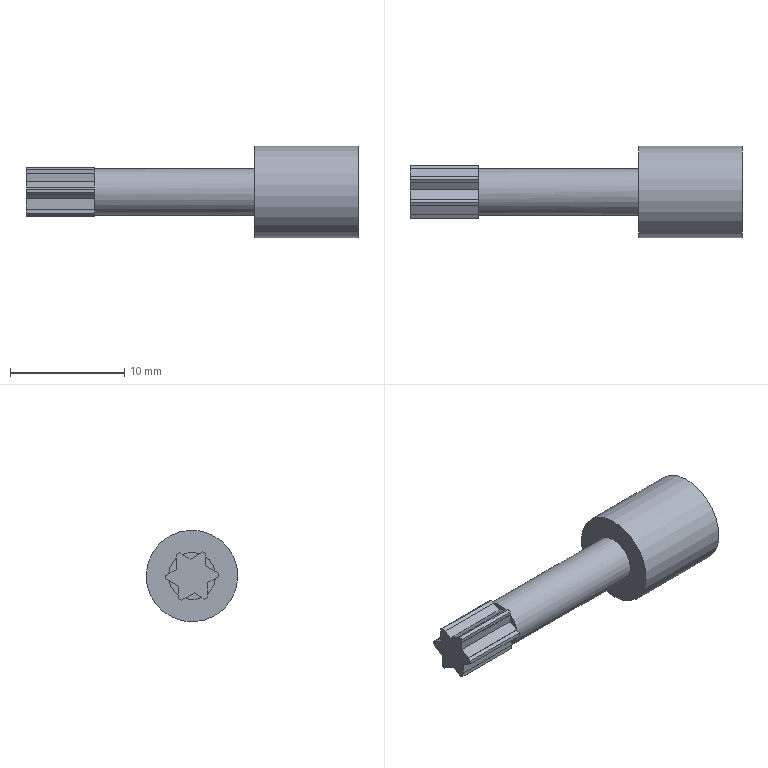Part | STEP file | Wytnij-wyci_gni_cie5 | 1 solid | 52 faces | box 29 x 8 x 8 mm | volume 614.096 mm3 | plane 42 | cylinder 10 | commonest cylinder face diameters 4.635 x6 4.9 x2 4.1 x1 8 x1